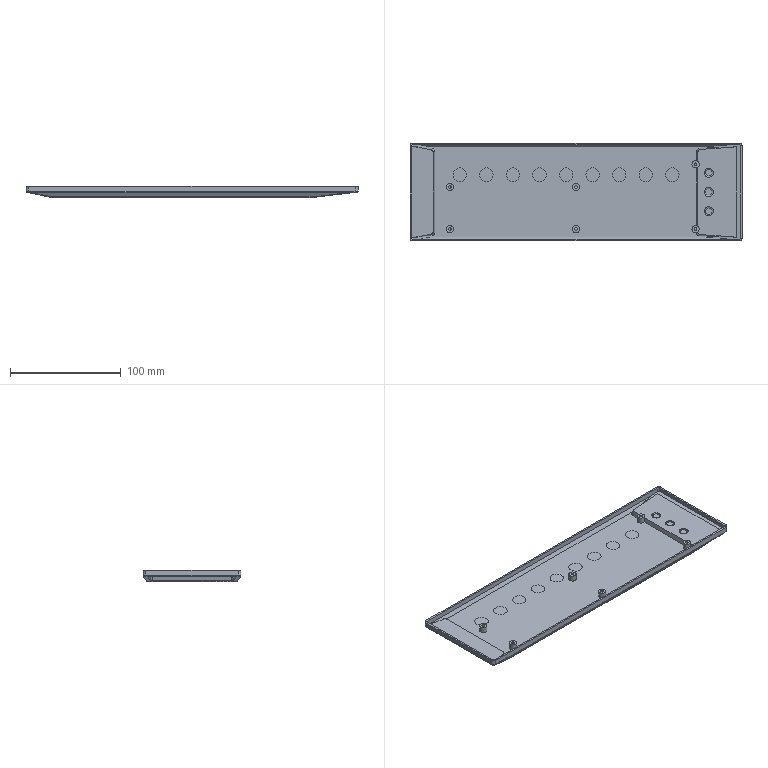NC program | NX | posted with a generic post | part box 300 x 88.5 x 10 mm
Lines 1 to 22 of 32249:
N10 G17 G21 G94 G90
(FLOOR_WALL , TOOL : D63)
N12 T01 M6
N14 G54
N16 G17 G0 G90 X-189.5 Y49.247 S6500 M3
N18 G43 Z30. H1
N20 Z3.
N22 G94 G1 Z0. F1250.
N24 X-186.5
N26 X186.5
N28 Y12.599
N30 X-186.5
N32 Y-24.05
N34 X186.5
N36 X189.5
N38 Z3.
N40 G0 Z30.
N42 M5